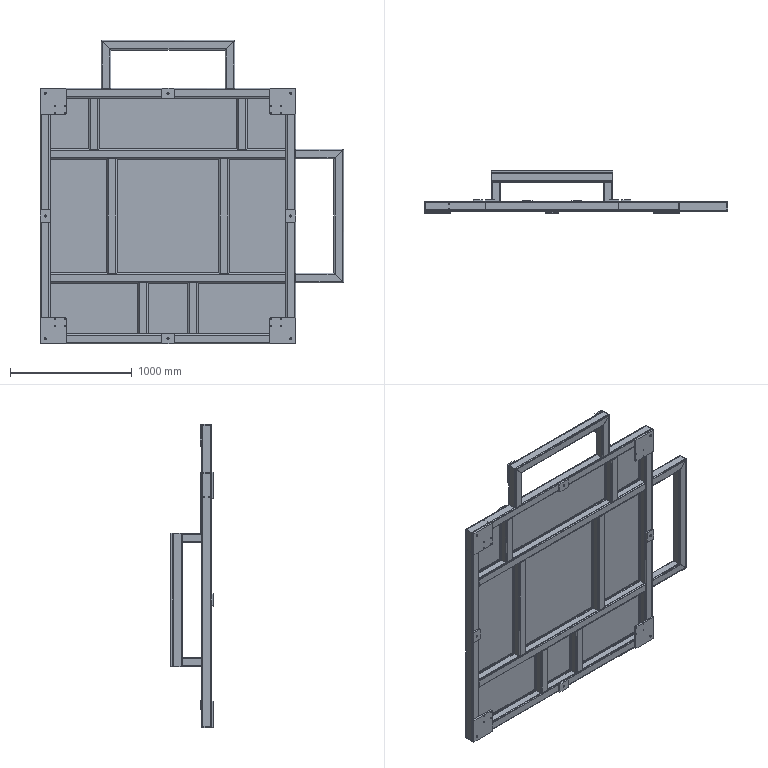Part | SolidWorks | features BaseBody 53 | 53 solids | 1194 faces | box 2495 x 350 x 2495 mm | volume 50017538 mm3 | plane 610 | cylinder 512 | spline 72 | commonest cylinder face diameters 10 x104 20 x104 8.5 x80 10.2 x44 6.8 x40 4 x36